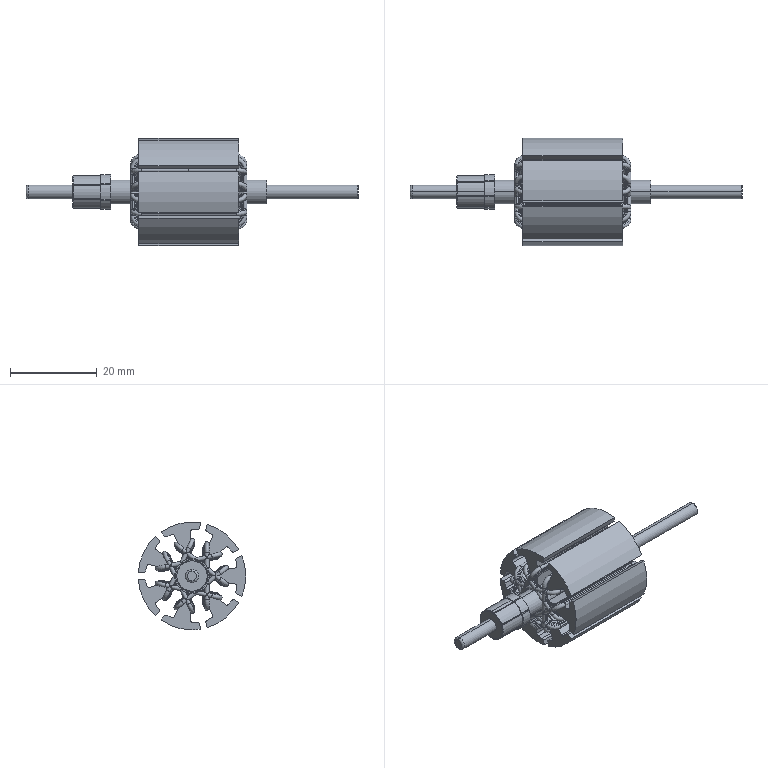Part | SolidWorks | features BaseBody 3 | 3 solids | 1238 faces | box 76.5 x 24.777 x 24.8 mm | volume 8261 mm3 | cylinder 896 | torus 256 | plane 86 | commonest cylinder face diameters 1 x852 6 x8 7.5 x8 8 x8 24.8 x8 3.11 x6